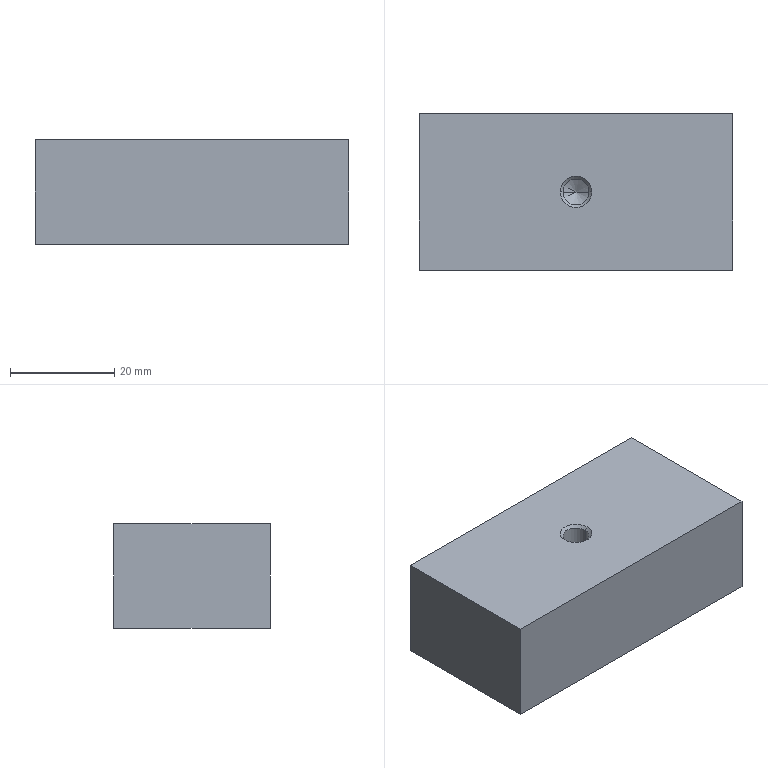Part | SolidWorks | features Extrusion 1, HoleWzd 1 | 1 solid | 12 faces | box 60 x 30 x 20 mm | volume 35693 mm3 | plane 6 | cone 4 | cylinder 2 | commonest cylinder face diameters 5 x2
STEP:
#1=CARTESIAN_POINT('',(717.5,45.,19.475));
#2=VERTEX_POINT('',#1);
#3=CARTESIAN_POINT('',(722.5,45.,19.475));
#4=VERTEX_POINT('',#3);
#5=CARTESIAN_POINT('',(720.,45.,19.475));
#6=DIRECTION('',(0.,0.,1.));
#7=DIRECTION('',(1.,0.,0.));
#8=AXIS2_PLACEMENT_3D('',#5,#6,#7);
#9=CIRCLE('',#8,2.5);
#10=EDGE_CURVE('',#2,#4,#9,.T.);
#11=ORIENTED_EDGE('',*,*,#10,.F.);
#12=CARTESIAN_POINT('',(716.975,45.,20.));
#13=VERTEX_POINT('',#12);
#14=CARTESIAN_POINT('',(716.975,45.,20.));
#15=DIRECTION('',(-0.7071,0.,0.7071));
#16=VECTOR('',#15,1000.);
#17=LINE('',#14,#16);
#18=EDGE_CURVE('',#2,#13,#17,.T.);
#19=ORIENTED_EDGE('',*,*,#18,.T.);
#20=CARTESIAN_POINT('',(723.025,45.,20.));
#21=VERTEX_POINT('',#20);
#22=CARTESIAN_POINT('',(720.,45.,20.));
#23=DIRECTION('',(0.,0.,1.));
#24=DIRECTION('',(1.,0.,0.));
#25=AXIS2_PLACEMENT_3D('',#22,#23,#24);
#26=CIRCLE('',#25,3.025);
#27=EDGE_CURVE('',#13,#21,#26,.T.);
#28=ORIENTED_EDGE('',*,*,#27,.T.);
#29=CARTESIAN_POINT('',(723.025,45.,20.));
#30=DIRECTION('',(0.7071,0.,0.7071));
#31=VECTOR('',#30,1000.);
#32=LINE('',#29,#31);
#33=EDGE_CURVE('',#4,#21,#32,.T.);
#34=ORIENTED_EDGE('',*,*,#33,.F.);
#35=EDGE_LOOP('',(#11,#19,#28,#34));
#36=FACE_OUTER_BOUND('',#35,.T.);
#37=CARTESIAN_POINT('',(720.,45.,20.));
#38=DIRECTION('',(0.,0.,1.));
#39=DIRECTION('',(1.,0.,0.));
#40=AXIS2_PLACEMENT_3D('',#37,#38,#39);
#41=CONICAL_SURFACE('',#40,3.025,0.7854);
#42=ADVANCED_FACE('',(#36),#41,.F.);
#43=CARTESIAN_POINT('',(717.5,45.,5.));
#44=VERTEX_POINT('',#43);
#45=CARTESIAN_POINT('',(722.5,45.,5.));
#46=VERTEX_POINT('',#45);
#47=CARTESIAN_POINT('',(720.,45.,5.));
#48=DIRECTION('',(0.,0.,1.));
#49=DIRECTION('',(1.,0.,0.));
#50=AXIS2_PLACEMENT_3D('',#47,#48,#49);
#51=CIRCLE('',#50,2.5);
#52=EDGE_CURVE('',#44,#46,#51,.T.);
#53=ORIENTED_EDGE('',*,*,#52,.F.);
#54=CARTESIAN_POINT('',(717.5,45.,20.));
#55=DIRECTION('',(0.,0.,1.));
#56=VECTOR('',#55,1000.);
#57=LINE('',#54,#56);
#58=EDGE_CURVE('',#44,#2,#57,.T.);
#59=ORIENTED_EDGE('',*,*,#58,.T.);
#60=ORIENTED_EDGE('',*,*,#10,.T.);
#61=CARTESIAN_POINT('',(722.5,45.,20.));
#62=DIRECTION('',(0.,0.,1.));
#63=VECTOR('',#62,1000.);
#64=LINE('',#61,#63);
#65=EDGE_CURVE('',#46,#4,#64,.T.);
#66=ORIENTED_EDGE('',*,*,#65,.F.);
#67=EDGE_LOOP('',(#53,#59,#60,#66));
#68=FACE_OUTER_BOUND('',#67,.T.);
#69=CARTESIAN_POINT('',(720.,45.,20.));
#70=DIRECTION('',(0.,0.,1.));
#71=DIRECTION('',(1.,0.,0.));
#72=AXIS2_PLACEMENT_3D('',#69,#70,#71);
#73=CYLINDRICAL_SURFACE('',#72,2.5);
#74=ADVANCED_FACE('',(#68),#73,.F.);
#75=CARTESIAN_POINT('',(720.,45.,3.498));
#76=VERTEX_POINT('',#75);
#77=CARTESIAN_POINT('',(722.5,45.,5.));
#78=DIRECTION('',(0.8572,0.,0.515));
#79=VECTOR('',#78,1000.);
#80=LINE('',#77,#79);
#81=EDGE_CURVE('',#76,#46,#80,.T.);
#82=ORIENTED_EDGE('',*,*,#81,.F.);
#83=CARTESIAN_POINT('',(717.5,45.,5.));
#84=DIRECTION('',(-0.8572,0.,0.515));
#85=VECTOR('',#84,1000.);
#86=LINE('',#83,#85);
#87=EDGE_CURVE('',#76,#44,#86,.T.);
#88=ORIENTED_EDGE('',*,*,#87,.T.);
#89=ORIENTED_EDGE('',*,*,#52,.T.);
#90=EDGE_LOOP('',(#82,#88,#89));
#91=FACE_OUTER_BOUND('',#90,.T.);
#92=CARTESIAN_POINT('',(720.,45.,5.));
#93=DIRECTION('',(0.,0.,1.));
#94=DIRECTION('',(1.,0.,0.));
#95=AXIS2_PLACEMENT_3D('',#92,#93,#94);
#96=CONICAL_SURFACE('',#95,2.5,1.03);
#97=ADVANCED_FACE('',(#91),#96,.F.);
#98=CARTESIAN_POINT('',(690.,60.,0.));
#99=VERTEX_POINT('',#98);
#100=CARTESIAN_POINT('',(690.,30.,0.));
#101=VERTEX_POINT('',#100);
#102=CARTESIAN_POINT('',(690.,30.,0.));
#103=DIRECTION('',(0.,-1.,0.));
#104=VECTOR('',#103,1000.);
#105=LINE('',#102,#104);
#106=EDGE_CURVE('',#99,#101,#105,.T.);
#107=ORIENTED_EDGE('',*,*,#106,.T.);
#108=CARTESIAN_POINT('',(690.,30.,20.));
#109=VERTEX_POINT('',#108);
#110=CARTESIAN_POINT('',(690.,30.,20.));
#111=DIRECTION('',(0.,0.,-1.));
#112=VECTOR('',#111,1000.);
#113=LINE('',#110,#112);
#114=EDGE_CURVE('',#109,#101,#113,.T.);
#115=ORIENTED_EDGE('',*,*,#114,.F.);
#116=CARTESIAN_POINT('',(690.,60.,20.));
#117=VERTEX_POINT('',#116);
#118=CARTESIAN_POINT('',(690.,30.,20.));
#119=DIRECTION('',(0.,-1.,0.));
#120=VECTOR('',#119,1000.);
#121=LINE('',#118,#120);
#122=EDGE_CURVE('',#117,#109,#121,.T.);
#123=ORIENTED_EDGE('',*,*,#122,.F.);
#124=CARTESIAN_POINT('',(690.,60.,20.));
#125=DIRECTION('',(0.,0.,-1.));
#126=VECTOR('',#125,1000.);
#127=LINE('',#124,#126);
#128=EDGE_CURVE('',#117,#99,#127,.T.);
#129=ORIENTED_EDGE('',*,*,#128,.T.);
#130=EDGE_LOOP('',(#107,#115,#123,#129));
#131=FACE_OUTER_BOUND('',#130,.T.);
#132=CARTESIAN_POINT('',(690.,30.,20.));
#133=DIRECTION('',(1.,0.,0.));
#134=DIRECTION('',(0.,0.,-1.));
#135=AXIS2_PLACEMENT_3D('',#132,#133,#134);
#136=PLANE('',#135);
#137=ADVANCED_FACE('',(#131),#136,.F.);
#138=CARTESIAN_POINT('',(750.,30.,0.));
#139=VERTEX_POINT('',#138);
#140=CARTESIAN_POINT('',(690.,30.,0.));
#141=DIRECTION('',(1.,0.,0.));
#142=VECTOR('',#141,1000.);
#143=LINE('',#140,#142);
#144=EDGE_CURVE('',#101,#139,#143,.T.);
#145=ORIENTED_EDGE('',*,*,#144,.T.);
#146=CARTESIAN_POINT('',(750.,30.,20.));
#147=VERTEX_POINT('',#146);
#148=CARTESIAN_POINT('',(750.,30.,20.));
#149=DIRECTION('',(0.,0.,-1.));
#150=VECTOR('',#149,1000.);
#151=LINE('',#148,#150);
#152=EDGE_CURVE('',#147,#139,#151,.T.);
#153=ORIENTED_EDGE('',*,*,#152,.F.);
#154=CARTESIAN_POINT('',(690.,30.,20.));
#155=DIRECTION('',(1.,0.,0.));
#156=VECTOR('',#155,1000.);
#157=LINE('',#154,#156);
#158=EDGE_CURVE('',#109,#147,#157,.T.);
#159=ORIENTED_EDGE('',*,*,#158,.F.);
#160=ORIENTED_EDGE('',*,*,#114,.T.);
#161=EDGE_LOOP('',(#145,#153,#159,#160));
#162=FACE_OUTER_BOUND('',#161,.T.);
#163=CARTESIAN_POINT('',(690.,30.,20.));
#164=DIRECTION('',(0.,1.,0.));
#165=DIRECTION('',(0.,0.,1.));
#166=AXIS2_PLACEMENT_3D('',#163,#164,#165);
#167=PLANE('',#166);
#168=ADVANCED_FACE('',(#162),#167,.F.);
#169=CARTESIAN_POINT('',(750.,60.,0.));
#170=VERTEX_POINT('',#169);
#171=CARTESIAN_POINT('',(750.,30.,0.));
#172=DIRECTION('',(0.,1.,0.));
#173=VECTOR('',#172,1000.);
#174=LINE('',#171,#173);
#175=EDGE_CURVE('',#139,#170,#174,.T.);
#176=ORIENTED_EDGE('',*,*,#175,.T.);
#177=CARTESIAN_POINT('',(750.,60.,20.));
#178=VERTEX_POINT('',#177);
#179=CARTESIAN_POINT('',(750.,60.,20.));
#180=DIRECTION('',(0.,0.,-1.));
#181=VECTOR('',#180,1000.);
#182=LINE('',#179,#181);
#183=EDGE_CURVE('',#178,#170,#182,.T.);
#184=ORIENTED_EDGE('',*,*,#183,.F.);
#185=CARTESIAN_POINT('',(750.,30.,20.));
#186=DIRECTION('',(0.,1.,0.));
#187=VECTOR('',#186,1000.);
#188=LINE('',#185,#187);
#189=EDGE_CURVE('',#147,#178,#188,.T.);
#190=ORIENTED_EDGE('',*,*,#189,.F.);
#191=ORIENTED_EDGE('',*,*,#152,.T.);
#192=EDGE_LOOP('',(#176,#184,#190,#191));
#193=FACE_OUTER_BOUND('',#192,.T.);
#194=CARTESIAN_POINT('',(750.,30.,20.));
#195=DIRECTION('',(-1.,0.,0.));
#196=DIRECTION('',(0.,0.,1.));
#197=AXIS2_PLACEMENT_3D('',#194,#195,#196);
#198=PLANE('',#197);
#199=ADVANCED_FACE('',(#193),#198,.F.);
#200=CARTESIAN_POINT('',(690.,60.,0.));
#201=DIRECTION('',(-1.,0.,0.));
#202=VECTOR('',#201,1000.);
#203=LINE('',#200,#202);
#204=EDGE_CURVE('',#170,#99,#203,.T.);
#205=ORIENTED_EDGE('',*,*,#204,.T.);
#206=ORIENTED_EDGE('',*,*,#128,.F.);
#207=CARTESIAN_POINT('',(690.,60.,20.));
#208=DIRECTION('',(-1.,0.,0.));
#209=VECTOR('',#208,1000.);
#210=LINE('',#207,#209);
#211=EDGE_CURVE('',#178,#117,#210,.T.);
#212=ORIENTED_EDGE('',*,*,#211,.F.);
#213=ORIENTED_EDGE('',*,*,#183,.T.);
#214=EDGE_LOOP('',(#205,#206,#212,#213));
#215=FACE_OUTER_BOUND('',#214,.T.);
#216=CARTESIAN_POINT('',(690.,60.,20.));
#217=DIRECTION('',(0.,-1.,0.));
#218=DIRECTION('',(0.,0.,-1.));
#219=AXIS2_PLACEMENT_3D('',#216,#217,#218);
#220=PLANE('',#219);
#221=ADVANCED_FACE('',(#215),#220,.F.);
#222=CARTESIAN_POINT('',(720.,45.,20.));
#223=DIRECTION('',(0.,0.,1.));
#224=DIRECTION('',(1.,0.,0.));
#225=AXIS2_PLACEMENT_3D('',#222,#223,#224);
#226=CIRCLE('',#225,3.025);
#227=EDGE_CURVE('',#21,#13,#226,.T.);
#228=ORIENTED_EDGE('',*,*,#227,.F.);
#229=ORIENTED_EDGE('',*,*,#27,.F.);
#230=EDGE_LOOP('',(#228,#229));
#231=FACE_BOUND('',#230,.T.);
#232=ORIENTED_EDGE('',*,*,#122,.T.);
#233=ORIENTED_EDGE('',*,*,#158,.T.);
#234=ORIENTED_EDGE('',*,*,#189,.T.);
#235=ORIENTED_EDGE('',*,*,#211,.T.);
#236=EDGE_LOOP('',(#232,#233,#234,#235));
#237=FACE_OUTER_BOUND('',#236,.T.);
#238=CARTESIAN_POINT('',(0.,0.,20.));
#239=DIRECTION('',(0.,0.,-1.));
#240=DIRECTION('',(-1.,0.,0.));
#241=AXIS2_PLACEMENT_3D('',#238,#239,#240);
#242=PLANE('',#241);
#243=ADVANCED_FACE('',(#231,#237),#242,.F.);
#244=ORIENTED_EDGE('',*,*,#106,.F.);
#245=ORIENTED_EDGE('',*,*,#204,.F.);
#246=ORIENTED_EDGE('',*,*,#175,.F.);
#247=ORIENTED_EDGE('',*,*,#144,.F.);
#248=EDGE_LOOP('',(#244,#245,#246,#247));
#249=FACE_OUTER_BOUND('',#248,.T.);
#250=CARTESIAN_POINT('',(0.,0.,0.));
#251=DIRECTION('',(0.,0.,-1.));
#252=DIRECTION('',(-1.,0.,0.));
#253=AXIS2_PLACEMENT_3D('',#250,#251,#252);
#254=PLANE('',#253);
#255=ADVANCED_FACE('',(#249),#254,.T.);
#256=ORIENTED_EDGE('',*,*,#87,.F.);
#257=ORIENTED_EDGE('',*,*,#81,.T.);
#258=CARTESIAN_POINT('',(720.,45.,5.));
#259=DIRECTION('',(0.,0.,1.));
#260=DIRECTION('',(1.,0.,0.));
#261=AXIS2_PLACEMENT_3D('',#258,#259,#260);
#262=CIRCLE('',#261,2.5);
#263=EDGE_CURVE('',#46,#44,#262,.T.);
#264=ORIENTED_EDGE('',*,*,#263,.T.);
#265=EDGE_LOOP('',(#256,#257,#264));
#266=FACE_OUTER_BOUND('',#265,.T.);
#267=CARTESIAN_POINT('',(720.,45.,5.));
#268=DIRECTION('',(0.,0.,1.));
#269=DIRECTION('',(1.,0.,0.));
#270=AXIS2_PLACEMENT_3D('',#267,#268,#269);
#271=CONICAL_SURFACE('',#270,2.5,1.03);
#272=ADVANCED_FACE('',(#266),#271,.F.);
#273=ORIENTED_EDGE('',*,*,#58,.F.);
#274=ORIENTED_EDGE('',*,*,#263,.F.);
#275=ORIENTED_EDGE('',*,*,#65,.T.);
#276=CARTESIAN_POINT('',(720.,45.,19.475));
#277=DIRECTION('',(0.,0.,1.));
#278=DIRECTION('',(1.,0.,0.));
#279=AXIS2_PLACEMENT_3D('',#276,#277,#278);
#280=CIRCLE('',#279,2.5);
#281=EDGE_CURVE('',#4,#2,#280,.T.);
#282=ORIENTED_EDGE('',*,*,#281,.T.);
#283=EDGE_LOOP('',(#273,#274,#275,#282));
#284=FACE_OUTER_BOUND('',#283,.T.);
#285=CARTESIAN_POINT('',(720.,45.,20.));
#286=DIRECTION('',(0.,0.,1.));
#287=DIRECTION('',(1.,0.,0.));
#288=AXIS2_PLACEMENT_3D('',#285,#286,#287);
#289=CYLINDRICAL_SURFACE('',#288,2.5);
#290=ADVANCED_FACE('',(#284),#289,.F.);
#291=ORIENTED_EDGE('',*,*,#18,.F.);
#292=ORIENTED_EDGE('',*,*,#281,.F.);
#293=ORIENTED_EDGE('',*,*,#33,.T.);
#294=ORIENTED_EDGE('',*,*,#227,.T.);
#295=EDGE_LOOP('',(#291,#292,#293,#294));
#296=FACE_OUTER_BOUND('',#295,.T.);
#297=CARTESIAN_POINT('',(720.,45.,20.));
#298=DIRECTION('',(0.,0.,1.));
#299=DIRECTION('',(1.,0.,0.));
#300=AXIS2_PLACEMENT_3D('',#297,#298,#299);
#301=CONICAL_SURFACE('',#300,3.025,0.7854);
#302=ADVANCED_FACE('',(#296),#301,.F.);
#303=CLOSED_SHELL('',(#42,#74,#97,#137,#168,#199,#221,#243,#255,#272,#290,#302));
#304=MANIFOLD_SOLID_BREP('',#303);
#305=CARTESIAN_POINT('',(0.,0.,0.));
#306=DIRECTION('',(0.,0.,1.));
#307=DIRECTION('',(1.,0.,0.));
#308=AXIS2_PLACEMENT_3D('',#305,#306,#307);
#309=(LENGTH_UNIT()NAMED_UNIT(*)SI_UNIT(.MILLI.,.METRE.));
#310=UNCERTAINTY_MEASURE_WITH_UNIT(LENGTH_MEASURE(0.00001),#309,'','');
#311=(NAMED_UNIT(*)PLANE_ANGLE_UNIT()SI_UNIT($,.RADIAN.));
#312=(NAMED_UNIT(*)SI_UNIT($,.STERADIAN.)SOLID_ANGLE_UNIT());
#313=(GEOMETRIC_REPRESENTATION_CONTEXT(3)GLOBAL_UNCERTAINTY_ASSIGNED_CONTEXT((#310))GLOBAL_UNIT_ASSIGNED_CONTEXT((#309,#311,#312))REPRESENTATION_CONTEXT('',''));
#314=ADVANCED_BREP_SHAPE_REPRESENTATION('',(#304,#308),#313);